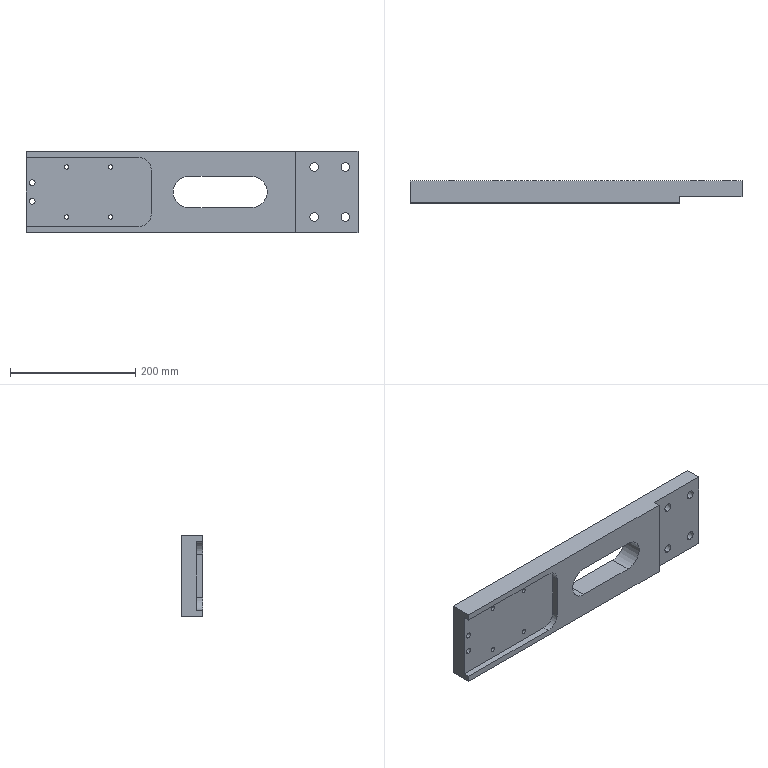Part | STEP file | fixing plate_default | 1 solid | 64 faces | box 530 x 35 x 130 mm | volume 1787786 mm3 | cylinder 36 | plane 20 | cone 8 | commonest cylinder face diameters 6.8 x8 13.5 x8 20 x8 9 x4 15 x4 40 x2